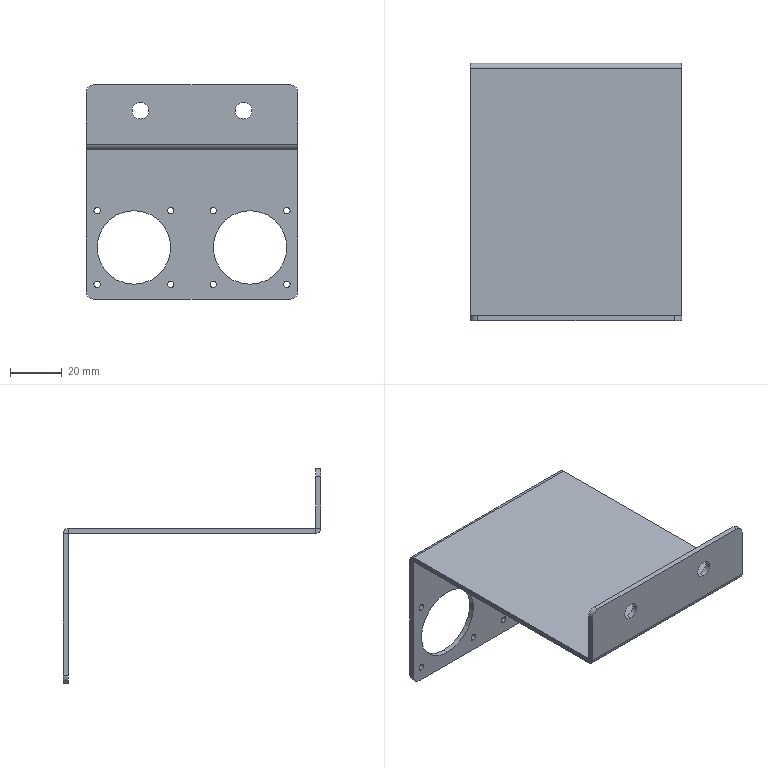Part | STEP file | Connector fixing plate 2 | 1 solid | 50 faces | box 82 x 100 x 83 mm | volume 26763 mm3 | cylinder 32 | plane 18 | commonest cylinder face diameters 2.5 x16 6 x4 6.5 x4 28.5 x4 0.02 x2 4.02 x2